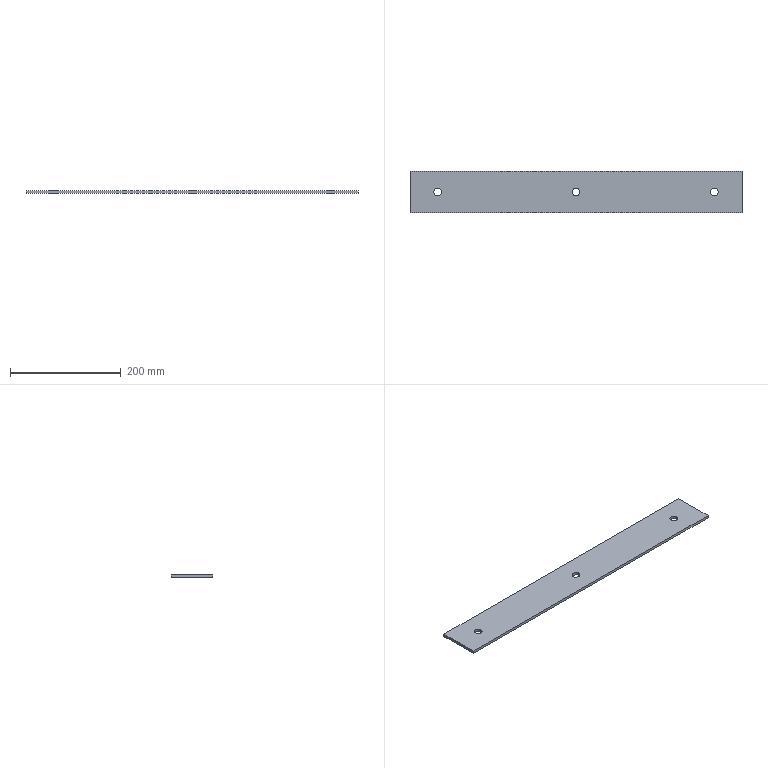Part | SolidWorks | features MoveFace 2, BaseBody 1 | 1 solid | 12 faces | box 600 x 75 x 5 mm | volume 222691 mm3 | cylinder 6 | plane 6 | commonest cylinder face diameters 14 x6
STEP:
#1=CARTESIAN_POINT('',(-7.,0.,0.));
#2=VERTEX_POINT('',#1);
#3=CARTESIAN_POINT('',(7.,0.,0.));
#4=VERTEX_POINT('',#3);
#5=CARTESIAN_POINT('',(0.,0.,0.));
#6=DIRECTION('',(0.,0.,1.));
#7=DIRECTION('',(1.,0.,0.));
#8=AXIS2_PLACEMENT_3D('',#5,#6,#7);
#9=CIRCLE('',#8,7.);
#10=EDGE_CURVE('',#2,#4,#9,.T.);
#11=ORIENTED_EDGE('',*,*,#10,.F.);
#12=CARTESIAN_POINT('',(-7.,0.,5.));
#13=VERTEX_POINT('',#12);
#14=CARTESIAN_POINT('',(-7.,0.,-5.));
#15=DIRECTION('',(0.,0.,1.));
#16=VECTOR('',#15,1000.);
#17=LINE('',#14,#16);
#18=EDGE_CURVE('',#2,#13,#17,.T.);
#19=ORIENTED_EDGE('',*,*,#18,.T.);
#20=CARTESIAN_POINT('',(7.,0.,5.));
#21=VERTEX_POINT('',#20);
#22=CARTESIAN_POINT('',(0.,0.,5.));
#23=DIRECTION('',(0.,0.,-1.));
#24=DIRECTION('',(1.,0.,0.));
#25=AXIS2_PLACEMENT_3D('',#22,#23,#24);
#26=CIRCLE('',#25,7.);
#27=EDGE_CURVE('',#21,#13,#26,.T.);
#28=ORIENTED_EDGE('',*,*,#27,.F.);
#29=CARTESIAN_POINT('',(7.,0.,-5.));
#30=DIRECTION('',(0.,0.,1.));
#31=VECTOR('',#30,1000.);
#32=LINE('',#29,#31);
#33=EDGE_CURVE('',#4,#21,#32,.T.);
#34=ORIENTED_EDGE('',*,*,#33,.F.);
#35=EDGE_LOOP('',(#11,#19,#28,#34));
#36=FACE_OUTER_BOUND('',#35,.T.);
#37=CARTESIAN_POINT('',(0.,0.,-5.));
#38=DIRECTION('',(0.,0.,1.));
#39=DIRECTION('',(1.,0.,0.));
#40=AXIS2_PLACEMENT_3D('',#37,#38,#39);
#41=CYLINDRICAL_SURFACE('',#40,7.);
#42=ADVANCED_FACE('',(#36),#41,.F.);
#43=CARTESIAN_POINT('',(-257.,0.,0.));
#44=VERTEX_POINT('',#43);
#45=CARTESIAN_POINT('',(-243.,0.,0.));
#46=VERTEX_POINT('',#45);
#47=CARTESIAN_POINT('',(-250.,0.,0.));
#48=DIRECTION('',(0.,0.,1.));
#49=DIRECTION('',(1.,0.,0.));
#50=AXIS2_PLACEMENT_3D('',#47,#48,#49);
#51=CIRCLE('',#50,7.);
#52=EDGE_CURVE('',#44,#46,#51,.T.);
#53=ORIENTED_EDGE('',*,*,#52,.F.);
#54=CARTESIAN_POINT('',(-257.,0.,5.));
#55=VERTEX_POINT('',#54);
#56=CARTESIAN_POINT('',(-257.,0.,-5.));
#57=DIRECTION('',(0.,0.,1.));
#58=VECTOR('',#57,1000.);
#59=LINE('',#56,#58);
#60=EDGE_CURVE('',#44,#55,#59,.T.);
#61=ORIENTED_EDGE('',*,*,#60,.T.);
#62=CARTESIAN_POINT('',(-243.,0.,5.));
#63=VERTEX_POINT('',#62);
#64=CARTESIAN_POINT('',(-250.,0.,5.));
#65=DIRECTION('',(0.,0.,-1.));
#66=DIRECTION('',(1.,0.,0.));
#67=AXIS2_PLACEMENT_3D('',#64,#65,#66);
#68=CIRCLE('',#67,7.);
#69=EDGE_CURVE('',#63,#55,#68,.T.);
#70=ORIENTED_EDGE('',*,*,#69,.F.);
#71=CARTESIAN_POINT('',(-243.,0.,-5.));
#72=DIRECTION('',(0.,0.,1.));
#73=VECTOR('',#72,1000.);
#74=LINE('',#71,#73);
#75=EDGE_CURVE('',#46,#63,#74,.T.);
#76=ORIENTED_EDGE('',*,*,#75,.F.);
#77=EDGE_LOOP('',(#53,#61,#70,#76));
#78=FACE_OUTER_BOUND('',#77,.T.);
#79=CARTESIAN_POINT('',(-250.,0.,-5.));
#80=DIRECTION('',(0.,0.,1.));
#81=DIRECTION('',(1.,0.,0.));
#82=AXIS2_PLACEMENT_3D('',#79,#80,#81);
#83=CYLINDRICAL_SURFACE('',#82,7.);
#84=ADVANCED_FACE('',(#78),#83,.F.);
#85=CARTESIAN_POINT('',(243.,0.,0.));
#86=VERTEX_POINT('',#85);
#87=CARTESIAN_POINT('',(257.,0.,0.));
#88=VERTEX_POINT('',#87);
#89=CARTESIAN_POINT('',(250.,0.,0.));
#90=DIRECTION('',(0.,0.,1.));
#91=DIRECTION('',(1.,0.,0.));
#92=AXIS2_PLACEMENT_3D('',#89,#90,#91);
#93=CIRCLE('',#92,7.);
#94=EDGE_CURVE('',#86,#88,#93,.T.);
#95=ORIENTED_EDGE('',*,*,#94,.F.);
#96=CARTESIAN_POINT('',(243.,0.,5.));
#97=VERTEX_POINT('',#96);
#98=CARTESIAN_POINT('',(243.,0.,-5.));
#99=DIRECTION('',(0.,0.,1.));
#100=VECTOR('',#99,1000.);
#101=LINE('',#98,#100);
#102=EDGE_CURVE('',#86,#97,#101,.T.);
#103=ORIENTED_EDGE('',*,*,#102,.T.);
#104=CARTESIAN_POINT('',(257.,0.,5.));
#105=VERTEX_POINT('',#104);
#106=CARTESIAN_POINT('',(250.,0.,5.));
#107=DIRECTION('',(0.,0.,-1.));
#108=DIRECTION('',(1.,0.,0.));
#109=AXIS2_PLACEMENT_3D('',#106,#107,#108);
#110=CIRCLE('',#109,7.);
#111=EDGE_CURVE('',#105,#97,#110,.T.);
#112=ORIENTED_EDGE('',*,*,#111,.F.);
#113=CARTESIAN_POINT('',(257.,0.,-5.));
#114=DIRECTION('',(0.,0.,1.));
#115=VECTOR('',#114,1000.);
#116=LINE('',#113,#115);
#117=EDGE_CURVE('',#88,#105,#116,.T.);
#118=ORIENTED_EDGE('',*,*,#117,.F.);
#119=EDGE_LOOP('',(#95,#103,#112,#118));
#120=FACE_OUTER_BOUND('',#119,.T.);
#121=CARTESIAN_POINT('',(250.,0.,-5.));
#122=DIRECTION('',(0.,0.,1.));
#123=DIRECTION('',(1.,0.,0.));
#124=AXIS2_PLACEMENT_3D('',#121,#122,#123);
#125=CYLINDRICAL_SURFACE('',#124,7.);
#126=ADVANCED_FACE('',(#120),#125,.F.);
#127=CARTESIAN_POINT('',(-300.,37.5,5.));
#128=VERTEX_POINT('',#127);
#129=CARTESIAN_POINT('',(-300.,-37.5,5.));
#130=VERTEX_POINT('',#129);
#131=CARTESIAN_POINT('',(-300.,0.,5.));
#132=DIRECTION('',(0.,-1.,0.));
#133=VECTOR('',#132,1000.);
#134=LINE('',#131,#133);
#135=EDGE_CURVE('',#128,#130,#134,.T.);
#136=ORIENTED_EDGE('',*,*,#135,.T.);
#137=CARTESIAN_POINT('',(300.,-37.5,5.));
#138=VERTEX_POINT('',#137);
#139=CARTESIAN_POINT('',(0.,-37.5,5.));
#140=DIRECTION('',(1.,0.,0.));
#141=VECTOR('',#140,1000.);
#142=LINE('',#139,#141);
#143=EDGE_CURVE('',#130,#138,#142,.T.);
#144=ORIENTED_EDGE('',*,*,#143,.T.);
#145=CARTESIAN_POINT('',(300.,37.5,5.));
#146=VERTEX_POINT('',#145);
#147=CARTESIAN_POINT('',(300.,0.,5.));
#148=DIRECTION('',(0.,1.,0.));
#149=VECTOR('',#148,1000.);
#150=LINE('',#147,#149);
#151=EDGE_CURVE('',#138,#146,#150,.T.);
#152=ORIENTED_EDGE('',*,*,#151,.T.);
#153=CARTESIAN_POINT('',(0.,37.5,5.));
#154=DIRECTION('',(-1.,0.,0.));
#155=VECTOR('',#154,1000.);
#156=LINE('',#153,#155);
#157=EDGE_CURVE('',#146,#128,#156,.T.);
#158=ORIENTED_EDGE('',*,*,#157,.T.);
#159=EDGE_LOOP('',(#136,#144,#152,#158));
#160=FACE_OUTER_BOUND('',#159,.T.);
#161=ORIENTED_EDGE('',*,*,#27,.T.);
#162=CARTESIAN_POINT('',(0.,0.,5.));
#163=DIRECTION('',(0.,0.,-1.));
#164=DIRECTION('',(1.,0.,0.));
#165=AXIS2_PLACEMENT_3D('',#162,#163,#164);
#166=CIRCLE('',#165,7.);
#167=EDGE_CURVE('',#13,#21,#166,.T.);
#168=ORIENTED_EDGE('',*,*,#167,.T.);
#169=EDGE_LOOP('',(#161,#168));
#170=FACE_BOUND('',#169,.T.);
#171=ORIENTED_EDGE('',*,*,#69,.T.);
#172=CARTESIAN_POINT('',(-250.,0.,5.));
#173=DIRECTION('',(0.,0.,-1.));
#174=DIRECTION('',(1.,0.,0.));
#175=AXIS2_PLACEMENT_3D('',#172,#173,#174);
#176=CIRCLE('',#175,7.);
#177=EDGE_CURVE('',#55,#63,#176,.T.);
#178=ORIENTED_EDGE('',*,*,#177,.T.);
#179=EDGE_LOOP('',(#171,#178));
#180=FACE_BOUND('',#179,.T.);
#181=ORIENTED_EDGE('',*,*,#111,.T.);
#182=CARTESIAN_POINT('',(250.,0.,5.));
#183=DIRECTION('',(0.,0.,-1.));
#184=DIRECTION('',(1.,0.,0.));
#185=AXIS2_PLACEMENT_3D('',#182,#183,#184);
#186=CIRCLE('',#185,7.);
#187=EDGE_CURVE('',#97,#105,#186,.T.);
#188=ORIENTED_EDGE('',*,*,#187,.T.);
#189=EDGE_LOOP('',(#181,#188));
#190=FACE_BOUND('',#189,.T.);
#191=CARTESIAN_POINT('',(0.,0.,5.));
#192=DIRECTION('',(0.,0.,1.));
#193=DIRECTION('',(1.,0.,0.));
#194=AXIS2_PLACEMENT_3D('',#191,#192,#193);
#195=PLANE('',#194);
#196=ADVANCED_FACE('',(#160,#170,#180,#190),#195,.T.);
#197=CARTESIAN_POINT('',(300.,-37.5,0.));
#198=VERTEX_POINT('',#197);
#199=CARTESIAN_POINT('',(300.,-37.5,5.));
#200=DIRECTION('',(0.,0.,-1.));
#201=VECTOR('',#200,1000.);
#202=LINE('',#199,#201);
#203=EDGE_CURVE('',#138,#198,#202,.T.);
#204=ORIENTED_EDGE('',*,*,#203,.F.);
#205=ORIENTED_EDGE('',*,*,#143,.F.);
#206=CARTESIAN_POINT('',(-300.,-37.5,0.));
#207=VERTEX_POINT('',#206);
#208=CARTESIAN_POINT('',(-300.,-37.5,5.));
#209=DIRECTION('',(0.,0.,1.));
#210=VECTOR('',#209,1000.);
#211=LINE('',#208,#210);
#212=EDGE_CURVE('',#207,#130,#211,.T.);
#213=ORIENTED_EDGE('',*,*,#212,.F.);
#214=CARTESIAN_POINT('',(-360.,-37.5,0.));
#215=DIRECTION('',(-1.,0.,0.));
#216=VECTOR('',#215,1000.);
#217=LINE('',#214,#216);
#218=EDGE_CURVE('',#198,#207,#217,.T.);
#219=ORIENTED_EDGE('',*,*,#218,.F.);
#220=EDGE_LOOP('',(#204,#205,#213,#219));
#221=FACE_OUTER_BOUND('',#220,.T.);
#222=CARTESIAN_POINT('',(-360.,-37.5,5.));
#223=DIRECTION('',(0.,1.,0.));
#224=DIRECTION('',(0.,0.,1.));
#225=AXIS2_PLACEMENT_3D('',#222,#223,#224);
#226=PLANE('',#225);
#227=ADVANCED_FACE('',(#221),#226,.F.);
#228=ORIENTED_EDGE('',*,*,#212,.T.);
#229=ORIENTED_EDGE('',*,*,#135,.F.);
#230=CARTESIAN_POINT('',(-300.,37.5,0.));
#231=VERTEX_POINT('',#230);
#232=CARTESIAN_POINT('',(-300.,37.5,5.));
#233=DIRECTION('',(0.,0.,1.));
#234=VECTOR('',#233,1000.);
#235=LINE('',#232,#234);
#236=EDGE_CURVE('',#231,#128,#235,.T.);
#237=ORIENTED_EDGE('',*,*,#236,.F.);
#238=CARTESIAN_POINT('',(-300.,37.5,0.));
#239=DIRECTION('',(0.,1.,0.));
#240=VECTOR('',#239,1000.);
#241=LINE('',#238,#240);
#242=EDGE_CURVE('',#207,#231,#241,.T.);
#243=ORIENTED_EDGE('',*,*,#242,.F.);
#244=EDGE_LOOP('',(#228,#229,#237,#243));
#245=FACE_OUTER_BOUND('',#244,.T.);
#246=CARTESIAN_POINT('',(-300.,37.5,5.));
#247=DIRECTION('',(1.,0.,0.));
#248=DIRECTION('',(0.,0.,-1.));
#249=AXIS2_PLACEMENT_3D('',#246,#247,#248);
#250=PLANE('',#249);
#251=ADVANCED_FACE('',(#245),#250,.F.);
#252=ORIENTED_EDGE('',*,*,#236,.T.);
#253=ORIENTED_EDGE('',*,*,#157,.F.);
#254=CARTESIAN_POINT('',(300.,37.5,0.));
#255=VERTEX_POINT('',#254);
#256=CARTESIAN_POINT('',(300.,37.5,5.));
#257=DIRECTION('',(0.,0.,1.));
#258=VECTOR('',#257,1000.);
#259=LINE('',#256,#258);
#260=EDGE_CURVE('',#255,#146,#259,.T.);
#261=ORIENTED_EDGE('',*,*,#260,.F.);
#262=CARTESIAN_POINT('',(-360.,37.5,0.));
#263=DIRECTION('',(1.,0.,0.));
#264=VECTOR('',#263,1000.);
#265=LINE('',#262,#264);
#266=EDGE_CURVE('',#231,#255,#265,.T.);
#267=ORIENTED_EDGE('',*,*,#266,.F.);
#268=EDGE_LOOP('',(#252,#253,#261,#267));
#269=FACE_OUTER_BOUND('',#268,.T.);
#270=CARTESIAN_POINT('',(-360.,37.5,5.));
#271=DIRECTION('',(0.,-1.,0.));
#272=DIRECTION('',(0.,0.,-1.));
#273=AXIS2_PLACEMENT_3D('',#270,#271,#272);
#274=PLANE('',#273);
#275=ADVANCED_FACE('',(#269),#274,.F.);
#276=ORIENTED_EDGE('',*,*,#260,.T.);
#277=ORIENTED_EDGE('',*,*,#151,.F.);
#278=ORIENTED_EDGE('',*,*,#203,.T.);
#279=CARTESIAN_POINT('',(300.,37.5,0.));
#280=DIRECTION('',(0.,-1.,0.));
#281=VECTOR('',#280,1000.);
#282=LINE('',#279,#281);
#283=EDGE_CURVE('',#255,#198,#282,.T.);
#284=ORIENTED_EDGE('',*,*,#283,.F.);
#285=EDGE_LOOP('',(#276,#277,#278,#284));
#286=FACE_OUTER_BOUND('',#285,.T.);
#287=CARTESIAN_POINT('',(300.,37.5,5.));
#288=DIRECTION('',(-1.,0.,0.));
#289=DIRECTION('',(0.,0.,1.));
#290=AXIS2_PLACEMENT_3D('',#287,#288,#289);
#291=PLANE('',#290);
#292=ADVANCED_FACE('',(#286),#291,.F.);
#293=ORIENTED_EDGE('',*,*,#18,.F.);
#294=CARTESIAN_POINT('',(0.,0.,0.));
#295=DIRECTION('',(0.,0.,1.));
#296=DIRECTION('',(1.,0.,0.));
#297=AXIS2_PLACEMENT_3D('',#294,#295,#296);
#298=CIRCLE('',#297,7.);
#299=EDGE_CURVE('',#4,#2,#298,.T.);
#300=ORIENTED_EDGE('',*,*,#299,.F.);
#301=ORIENTED_EDGE('',*,*,#33,.T.);
#302=ORIENTED_EDGE('',*,*,#167,.F.);
#303=EDGE_LOOP('',(#293,#300,#301,#302));
#304=FACE_OUTER_BOUND('',#303,.T.);
#305=CARTESIAN_POINT('',(0.,0.,-5.));
#306=DIRECTION('',(0.,0.,1.));
#307=DIRECTION('',(1.,0.,0.));
#308=AXIS2_PLACEMENT_3D('',#305,#306,#307);
#309=CYLINDRICAL_SURFACE('',#308,7.);
#310=ADVANCED_FACE('',(#304),#309,.F.);
#311=ORIENTED_EDGE('',*,*,#60,.F.);
#312=CARTESIAN_POINT('',(-250.,0.,0.));
#313=DIRECTION('',(0.,0.,1.));
#314=DIRECTION('',(1.,0.,0.));
#315=AXIS2_PLACEMENT_3D('',#312,#313,#314);
#316=CIRCLE('',#315,7.);
#317=EDGE_CURVE('',#46,#44,#316,.T.);
#318=ORIENTED_EDGE('',*,*,#317,.F.);
#319=ORIENTED_EDGE('',*,*,#75,.T.);
#320=ORIENTED_EDGE('',*,*,#177,.F.);
#321=EDGE_LOOP('',(#311,#318,#319,#320));
#322=FACE_OUTER_BOUND('',#321,.T.);
#323=CARTESIAN_POINT('',(-250.,0.,-5.));
#324=DIRECTION('',(0.,0.,1.));
#325=DIRECTION('',(1.,0.,0.));
#326=AXIS2_PLACEMENT_3D('',#323,#324,#325);
#327=CYLINDRICAL_SURFACE('',#326,7.);
#328=ADVANCED_FACE('',(#322),#327,.F.);
#329=ORIENTED_EDGE('',*,*,#102,.F.);
#330=CARTESIAN_POINT('',(250.,0.,0.));
#331=DIRECTION('',(0.,0.,1.));
#332=DIRECTION('',(1.,0.,0.));
#333=AXIS2_PLACEMENT_3D('',#330,#331,#332);
#334=CIRCLE('',#333,7.);
#335=EDGE_CURVE('',#88,#86,#334,.T.);
#336=ORIENTED_EDGE('',*,*,#335,.F.);
#337=ORIENTED_EDGE('',*,*,#117,.T.);
#338=ORIENTED_EDGE('',*,*,#187,.F.);
#339=EDGE_LOOP('',(#329,#336,#337,#338));
#340=FACE_OUTER_BOUND('',#339,.T.);
#341=CARTESIAN_POINT('',(250.,0.,-5.));
#342=DIRECTION('',(0.,0.,1.));
#343=DIRECTION('',(1.,0.,0.));
#344=AXIS2_PLACEMENT_3D('',#341,#342,#343);
#345=CYLINDRICAL_SURFACE('',#344,7.);
#346=ADVANCED_FACE('',(#340),#345,.F.);
#347=ORIENTED_EDGE('',*,*,#218,.T.);
#348=ORIENTED_EDGE('',*,*,#242,.T.);
#349=ORIENTED_EDGE('',*,*,#266,.T.);
#350=ORIENTED_EDGE('',*,*,#283,.T.);
#351=EDGE_LOOP('',(#347,#348,#349,#350));
#352=FACE_OUTER_BOUND('',#351,.T.);
#353=ORIENTED_EDGE('',*,*,#299,.T.);
#354=ORIENTED_EDGE('',*,*,#10,.T.);
#355=EDGE_LOOP('',(#353,#354));
#356=FACE_BOUND('',#355,.T.);
#357=ORIENTED_EDGE('',*,*,#317,.T.);
#358=ORIENTED_EDGE('',*,*,#52,.T.);
#359=EDGE_LOOP('',(#357,#358));
#360=FACE_BOUND('',#359,.T.);
#361=ORIENTED_EDGE('',*,*,#335,.T.);
#362=ORIENTED_EDGE('',*,*,#94,.T.);
#363=EDGE_LOOP('',(#361,#362));
#364=FACE_BOUND('',#363,.T.);
#365=CARTESIAN_POINT('',(0.,0.,0.));
#366=DIRECTION('',(0.,0.,1.));
#367=DIRECTION('',(1.,0.,0.));
#368=AXIS2_PLACEMENT_3D('',#365,#366,#367);
#369=PLANE('',#368);
#370=ADVANCED_FACE('',(#352,#356,#360,#364),#369,.F.);
#371=CLOSED_SHELL('',(#42,#84,#126,#196,#227,#251,#275,#292,#310,#328,#346,#370));
#372=MANIFOLD_SOLID_BREP('',#371);
#373=CARTESIAN_POINT('',(0.,0.,0.));
#374=DIRECTION('',(0.,0.,1.));
#375=DIRECTION('',(1.,0.,0.));
#376=AXIS2_PLACEMENT_3D('',#373,#374,#375);
#377=(LENGTH_UNIT()NAMED_UNIT(*)SI_UNIT(.MILLI.,.METRE.));
#378=UNCERTAINTY_MEASURE_WITH_UNIT(LENGTH_MEASURE(0.00001),#377,'','');
#379=(NAMED_UNIT(*)PLANE_ANGLE_UNIT()SI_UNIT($,.RADIAN.));
#380=(NAMED_UNIT(*)SI_UNIT($,.STERADIAN.)SOLID_ANGLE_UNIT());
#381=(GEOMETRIC_REPRESENTATION_CONTEXT(3)GLOBAL_UNCERTAINTY_ASSIGNED_CONTEXT((#378))GLOBAL_UNIT_ASSIGNED_CONTEXT((#377,#379,#380))REPRESENTATION_CONTEXT('',''));
#382=ADVANCED_BREP_SHAPE_REPRESENTATION('',(#372,#376),#381);